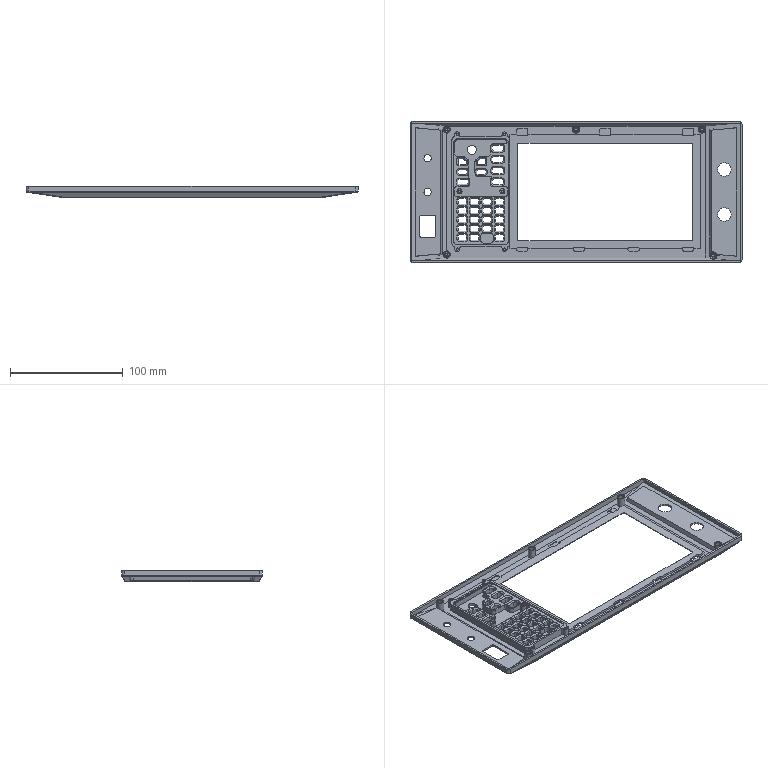NC program | NX | posted with a generic post | part box 295 x 125 x 10 mm
Lines 11539 to 12429 of 134431:
(HOLE_MILLING , TOOL : D4)
N23028 T04 M6
N23030 G54
N23032 G17 G0 G90 X-92.5 Y37.45 S9500 M3
N23034 G43 Z30. H4
N23036 Z-7.
N23038 G94 G3 X-91.875 Y36.825 R0.625 F1400.
N23040 X-91.25 Y37.45 R0.625
N23042 X-91.25 Y37.45 Z-7.4 I-1.25 J0.
N23044 X-91.25 Y37.45 Z-7.8 I-1.25 J0.
N23046 X-91.25 Y37.45 Z-8.2 I-1.25 J0.
N23048 X-91.25 Y37.45 Z-8.6 I-1.25 J0.
N23050 X-91.25 Y37.45 Z-9. I-1.25 J0.
N23052 X-91.25 Y37.45 Z-9.4 I-1.25 J0.
N23054 X-91.25 Y37.45 Z-9.8 I-1.25 J0.
N23056 X-93.75 Y37.45 Z-10. I-1.25 J0.
N23058 X-92.827 Y36.181 R1.334
N23060 X-91.326 Y36.665 R1.348
N23062 X-91.334 Y38.383 R1.44
N23064 X-93.103 Y38.905 R1.545
N23066 X-94.149 Y37.306 R1.602
N23068 X-92.839 Y35.746 R1.708
N23070 X-90.85 Y36.626 R1.798
N23072 X-91.156 Y38.794 R1.821
N23074 X-93.844 Y38.794 R1.9
N23076 X-91.156 Y38.794 R-1.9
N23078 X-92.5 Y38.794 R0.95
N23080 X-92.5 Y37.45 R0.95
N23082 G0 Z30.
N23084 X-131.817 Y30.
N23086 Z-3.769
N23088 G3 X-131.242 Y29.425 R0.575
N23090 X-130.667 Y30. R0.575
N23092 X-130.667 Y30. Z-4.169 I-1.15 J0.
N23094 X-130.667 Y30. Z-4.569 I-1.15 J0.
N23096 X-130.667 Y30. Z-4.969 I-1.15 J0.
N23098 X-130.667 Y30. Z-5.369 I-1.15 J0.
N23100 X-130.667 Y30. Z-5.769 I-1.15 J0.
N23102 X-131.817 Y31.15 R1.15
N23104 X-130.667 Y30. R-1.15
N23106 X-131.242 Y30.575 R0.575
N23108 X-131.817 Y30. R0.575
N23110 G0 Z30.
N23112 Y0.
N23114 Z-3.769
N23116 G3 X-131.242 Y-0.575 R0.575
N23118 X-130.667 Y0. R0.575
N23120 X-130.667 Y0. Z-4.169 I-1.15 J0.
N23122 X-130.667 Y0. Z-4.569 I-1.15 J0.
N23124 X-130.667 Y0. Z-4.969 I-1.15 J0.
N23126 X-130.667 Y0. Z-5.369 I-1.15 J0.
N23128 X-130.667 Y0. Z-5.769 I-1.15 J0.
N23130 X-131.817 Y1.15 R1.15
N23132 X-130.667 Y0. R-1.15
N23134 X-131.242 Y0.575 R0.575
N23136 X-131.817 Y0. R0.575
N23138 G0 Z30.
N23140 X131.817 Y20.
N23142 Z-3.769
N23144 G3 X132.442 Y19.375 R0.625
N23146 X133.067 Y20. R0.625
N23148 X133.067 Y20. Z-4.169 I-1.25 J0.
N23150 X133.067 Y20. Z-4.569 I-1.25 J0.
N23152 X133.067 Y20. Z-4.969 I-1.25 J0.
N23154 X133.067 Y20. Z-5.369 I-1.25 J0.
N23156 X133.067 Y20. Z-5.769 I-1.25 J0.
N23158 X131.862 Y21.318 R1.323
N23160 X130.398 Y20.241 R1.372
N23162 X131.41 Y18.522 R1.472
N23164 X133.354 Y19.462 R1.593
N23166 X132.543 Y21.562 R1.661
N23168 X130.226 Y20.879 R1.783
N23170 X130.734 Y18.424 R1.851
N23172 X133.386 Y18.749 R1.972
N23174 X133.278 Y21.51 R2.04
N23176 X130.353 Y21.638 R2.161
N23178 X129.972 Y18.642 R2.23
N23180 X133.086 Y17.98 R2.351
N23182 X134.031 Y21.116 R2.419
N23184 X130.831 Y22.379 R2.54
N23186 X129.266 Y19.213 R2.608
N23188 X132.432 Y17.305 R2.729
N23190 X134.651 Y20.375 R2.798
N23192 X131.651 Y22.949 R2.919
N23194 X128.771 Y20.11 R2.987
N23196 X131.465 Y16.877 R3.108
N23198 X134.987 Y19.345 R3.176
N23200 X132.739 Y23.202 R3.297
N23202 X128.624 Y21.245 R3.366
N23204 X130.289 Y16.827 R3.487
N23206 X134.919 Y18.142 R3.555
N23208 X133.964 Y23.026 R3.676
N23210 X128.846 Y22.427 R3.776
N23212 X129.059 Y17.242 R3.829
N23214 X134.575 Y17.242 R3.9
N23216 X129.059 Y17.242 R-3.9
N23218 X131.817 Y17.242 R1.95
N23220 X131.817 Y20. R1.95
N23222 G0 Z30.
N23224 Y-20.
N23226 Z-3.769
N23228 G3 X132.442 Y-20.625 R0.625
N23230 X133.067 Y-20. R0.625
N23232 X133.067 Y-20. Z-4.169 I-1.25 J0.
N23234 X133.067 Y-20. Z-4.569 I-1.25 J0.
N23236 X133.067 Y-20. Z-4.969 I-1.25 J0.
N23238 X133.067 Y-20. Z-5.369 I-1.25 J0.
N23240 X133.067 Y-20. Z-5.769 I-1.25 J0.
N23242 X131.862 Y-18.682 R1.323
N23244 X130.398 Y-19.759 R1.372
N23246 X131.41 Y-21.478 R1.472
N23248 X133.354 Y-20.538 R1.593
N23250 X132.543 Y-18.438 R1.661
N23252 X130.226 Y-19.121 R1.783
N23254 X130.734 Y-21.576 R1.851
N23256 X133.386 Y-21.251 R1.972
N23258 X133.278 Y-18.49 R2.04
N23260 X130.353 Y-18.362 R2.161
N23262 X129.972 Y-21.358 R2.23
N23264 X133.086 Y-22.02 R2.351
N23266 X134.031 Y-18.884 R2.419
N23268 X130.831 Y-17.621 R2.54
N23270 X129.266 Y-20.787 R2.608
N23272 X132.432 Y-22.695 R2.729
N23274 X134.651 Y-19.625 R2.798
N23276 X131.651 Y-17.051 R2.919
N23278 X128.771 Y-19.89 R2.987
N23280 X131.465 Y-23.123 R3.108
N23282 X134.987 Y-20.655 R3.176
N23284 X132.739 Y-16.798 R3.297
N23286 X128.624 Y-18.755 R3.366
N23288 X130.289 Y-23.173 R3.487
N23290 X134.919 Y-21.858 R3.555
N23292 X133.964 Y-16.974 R3.676
N23294 X128.846 Y-17.573 R3.776
N23296 X129.059 Y-22.758 R3.829
N23298 X134.575 Y-22.758 R3.9
N23300 X129.059 Y-22.758 R-3.9
N23302 X131.817 Y-22.758 R1.95
N23304 X131.817 Y-20. R1.95
N23306 G0 Z30.
(HOLE_MILLING_COPY , TOOL : D4)
N23308 X-92.5 Y37.45
N23310 Z-7.
N23312 G3 X-91.5 Y36.45 R1. F1000.
N23314 X-90.5 Y37.45 R1.
N23316 X-90.5 Y37.45 Z-9. I-2. J0.
N23318 X-94.5 Y37.45 Z-10. I-2. J0.
N23320 X-92.5 Y35.45 R2.
N23322 X-94.5 Y37.45 R-2.
N23324 X-93.5 Y36.45 R1.
N23326 X-92.5 Y37.45 R1.
N23328 G0 Z30.
N23330 X-131.817 Y30.
N23332 Z-3.769
N23334 G3 X-131.192 Y29.375 R0.625
N23336 X-130.567 Y30. R0.625
N23338 X-130.567 Y30. Z-5.769 I-1.25 J0.
N23340 X-131.817 Y31.25 R1.25
N23342 X-130.567 Y30. R-1.25
N23344 X-131.192 Y30.625 R0.625
N23346 X-131.817 Y30. R0.625
N23348 G0 Z30.
N23350 Y0.
N23352 Z-3.769
N23354 G3 X-131.192 Y-0.625 R0.625
N23356 X-130.567 Y0. R0.625
N23358 X-130.567 Y0. Z-5.769 I-1.25 J0.
N23360 X-131.817 Y1.25 R1.25
N23362 X-130.567 Y0. R-1.25
N23364 X-131.192 Y0.625 R0.625
N23366 X-131.817 Y0. R0.625
N23368 G0 Z30.
N23370 X131.817 Y20.
N23372 Z-3.769
N23374 G1 X132.202 Y19.187
N23376 G3 X135.817 Y20. R1.899
N23378 X135.817 Y20. Z-5.769 I-4. J0.
N23380 X131.817 Y24. R4.
N23382 X135.817 Y20. R-4.
N23384 X132.202 Y20.813 R1.899
N23386 G1 X131.817 Y20.
N23388 G0 Z30.
N23390 Y-20.
N23392 Z-3.769
N23394 G1 X132.202 Y-20.813
N23396 G3 X135.817 Y-20. R1.899
N23398 X135.817 Y-20. Z-5.769 I-4. J0.
N23400 X131.817 Y-16. R4.
N23402 X135.817 Y-20. R-4.
N23404 X132.202 Y-19.187 R1.899
N23406 G1 X131.817 Y-20.
N23408 G0 Z30.
(CAVITY_MILL_COPY_COPY , TOOL : D4)
N23410 X114.594 Y-58.2
N23412 Z0.625
N23414 G1 Z-0.375
N23416 X114.768 Y-58.5
N23418 G3 X115.634 Y-59. R1.
N23420 G1 X117.383 F1650.
N23422 G2 X116.837 Y-57.451 R5.25
N23424 G3 X116.188 Y-56.69 R1.
N23426 G1 X115.951 Y-56.606
N23428 Z0.625
N23430 G0 Z30.
N23432 X114.594 Y-58.2
N23434 Z0.25
N23436 G1 Z-0.75 F1000.
N23438 X114.768 Y-58.5
N23440 G3 X115.634 Y-59. R1.
N23442 G1 X117.383 F1650.
N23444 G2 X116.837 Y-57.451 R5.25
N23446 G3 X116.188 Y-56.69 R1.
N23448 G1 X115.951 Y-56.606
N23450 Z0.25
N23452 G0 X114.594 Y-58.2 Z-0.125
N23454 G1 Z-1.125 F1000.
N23456 X114.768 Y-58.5
N23458 G3 X115.634 Y-59. R1.
N23460 G1 X117.383 F1650.
N23462 G2 X116.837 Y-57.451 R5.25
N23464 G3 X116.188 Y-56.69 R1.
N23466 G1 X115.951 Y-56.606
N23468 Z-0.125
N23470 G0 X114.594 Y-58.2 Z-0.5
N23472 G1 Z-1.5 F1000.
N23474 X114.768 Y-58.5
N23476 G3 X115.634 Y-59. R1.
N23478 G1 X117.383 F1650.
N23480 G2 X116.837 Y-57.451 R5.25
N23482 G3 X116.188 Y-56.69 R1.
N23484 G1 X115.951 Y-56.606
N23486 Z-0.5
N23488 G0 X114.594 Y-58.2 Z-0.833
N23490 G1 Z-1.833 F1000.
N23492 X114.768 Y-58.5
N23494 G3 X115.634 Y-59. R1.
N23496 G1 X117.383 F1650.
N23498 G2 X116.837 Y-57.451 R5.25
N23500 G3 X116.188 Y-56.69 R1.
N23502 G1 X115.951 Y-56.606
N23504 Z-0.833
N23506 G0 X114.594 Y-58.2 Z-1.167
N23508 G1 Z-2.167 F1000.
N23510 X114.768 Y-58.5
N23512 G3 X115.634 Y-59. R1.
N23514 G1 X117.383 F1650.
N23516 G2 X116.837 Y-57.451 R5.25
N23518 G3 X116.188 Y-56.69 R1.
N23520 G1 X115.951 Y-56.606
N23522 Z-1.167
N23524 G0 X114.594 Y-58.2 Z-1.5
N23526 G1 Z-2.5 F1000.
N23528 X114.768 Y-58.5
N23530 G3 X115.634 Y-59. R1.
N23532 G1 X117.383 F1650.
N23534 G2 X116.837 Y-57.451 R5.25
N23536 G3 X116.188 Y-56.69 R1.
N23538 G1 X115.951 Y-56.606
N23540 Z-1.5
N23542 G0 X114.594 Y-58.2 Z-1.833
N23544 G1 Z-2.833 F1000.
N23546 X114.768 Y-58.5
N23548 G3 X115.634 Y-59. R1.
N23550 G1 X117.383 F1650.
N23552 G2 X116.837 Y-57.451 R5.25
N23554 G3 X116.188 Y-56.69 R1.
N23556 G1 X115.951 Y-56.606
N23558 Z-1.833
N23560 G0 X114.594 Y-58.2 Z-2.167
N23562 G1 Z-3.167 F1000.
N23564 X114.768 Y-58.5
N23566 G3 X115.634 Y-59. R1.
N23568 G1 X117.383 F1650.
N23570 G2 X116.837 Y-57.451 R5.25
N23572 G3 X116.188 Y-56.69 R1.
N23574 G1 X115.951 Y-56.606
N23576 Z-2.167
N23578 G0 X114.594 Y-58.2 Z-2.5
N23580 G1 Z-3.5 F1000.
N23582 X114.768 Y-58.5
N23584 G3 X115.634 Y-59. R1.
N23586 G1 X117.383 F1650.
N23588 G2 X116.837 Y-57.451 R5.25
N23590 G3 X116.188 Y-56.69 R1.
N23592 G1 X115.951 Y-56.606
N23594 Z-2.5
N23596 G0 X114.594 Y-58.2 Z-2.885
N23598 G1 Z-3.885 F1000.
N23600 X114.768 Y-58.5
N23602 G3 X115.634 Y-59. R1.
N23604 G1 X117.383 F1650.
N23606 G2 X116.837 Y-57.451 R5.25
N23608 G3 X116.188 Y-56.69 R1.
N23610 G1 X115.951 Y-56.606
N23612 Z-2.885
N23614 G0 X114.594 Y-58.2 Z-3.269
N23616 G1 Z-4.269 F1000.
N23618 X114.768 Y-58.5
N23620 G3 X115.634 Y-59. R1.
N23622 G1 X117.383 F1650.
N23624 G2 X116.837 Y-57.451 R5.25
N23626 G3 X116.188 Y-56.69 R1.
N23628 G1 X115.951 Y-56.606
N23630 Z-3.269
N23632 G0 X114.586 Y-58.166 Z-3.641
N23634 G1 Z-4.641 F1000.
N23636 X114.759 Y-58.466
N23638 G3 X115.625 Y-58.966 R1.
N23640 G1 X117.365 F1650.
N23642 G2 X116.832 Y-57.422 R5.25
N23644 G3 X116.187 Y-56.658 R1.
N23646 G1 X115.95 Y-56.572
N23648 Z-3.641
N23650 G0 X114.537 Y-57.943 Z-4.013
N23652 G1 Z-5.013 F1000.
N23654 X114.71 Y-58.243
N23656 G3 X115.576 Y-58.743 R1.
N23658 G1 X117.253 F1650.
N23660 G2 X116.801 Y-57.233 R5.25
N23662 G3 X116.185 Y-56.445 R1.
N23664 G1 X115.952 Y-56.351
N23666 Z-4.013
N23668 G0 X114.496 Y-57.72 Z-4.385
N23670 G1 Z-5.385 F1000.
N23672 X114.669 Y-58.02
N23674 G3 X115.535 Y-58.52 R1.
N23676 G1 X117.154 F1650.
N23678 G2 X116.778 Y-57.044 R5.25
N23680 G3 X116.191 Y-56.234 R1.
N23682 G1 X115.961 Y-56.131
N23684 Z-4.385
N23686 G0 X114.463 Y-57.497 Z-4.756
N23688 G1 Z-5.756 F1000.
N23690 X114.636 Y-57.797
N23692 G3 X115.502 Y-58.297 R1.
N23694 G1 X117.067 F1650.
N23696 G2 X116.762 Y-56.855 R5.25
N23698 G3 X116.205 Y-56.025 R1.
N23700 G1 X115.978 Y-55.914
N23702 Z-4.756
N23704 G0 X114.438 Y-57.274 Z-5.128
N23706 G1 Z-6.128 F1000.
N23708 X114.611 Y-57.574
N23710 G3 X115.477 Y-58.074 R1.
N23712 G1 X116.991 F1650.
N23714 G2 X116.753 Y-56.667 R5.25
N23716 G3 X116.225 Y-55.817 R1.
N23718 G1 X116.003 Y-55.698
N23720 Z-5.128
N23722 G0 X114.422 Y-57.052 Z-5.5
N23724 G1 Z-6.5 F1000.
N23726 X114.595 Y-57.352
N23728 G3 X115.461 Y-57.852 R1.
N23730 G1 X116.927 F1650.
N23732 G2 X116.75 Y-56.48 R5.25
N23734 G3 X116.253 Y-55.612 R1.
N23736 G1 X116.036 Y-55.485
N23738 Z-5.5
N23740 G0 X114.414 Y-56.851 Z-5.833
N23742 G1 Z-6.833 F1000.
N23744 X114.587 Y-57.151
N23746 G3 X115.453 Y-57.651 R1.
N23748 G1 X116.878 F1650.
N23750 G2 X116.753 Y-56.311 R5.25
N23752 G3 X116.285 Y-55.427 R1.
N23754 G1 X116.072 Y-55.293
N23756 Z-5.833
N23758 G0 X114.412 Y-56.651 Z-6.167
N23760 G1 Z-7.167 F1000.
N23762 X114.585 Y-56.951
N23764 G3 X115.451 Y-57.451 R1.
N23766 G1 X116.837 F1650.
N23768 G2 X116.762 Y-56.143 R5.25
N23770 G3 X116.322 Y-55.245 R1.
N23772 G1 X116.113 Y-55.104
N23774 Z-6.167
N23776 G0 X114.417 Y-56.452 Z-6.5
N23778 G1 Z-7.5 F1000.
N23780 X114.59 Y-56.752
N23782 G3 X115.456 Y-57.252 R1.
N23784 G1 X116.804 F1650.
N23786 G2 X116.776 Y-55.977 R5.25
N23788 G3 X116.365 Y-55.065 R1.
N23790 G1 X116.16 Y-54.918
N23792 Z-6.5
N23794 G0 X114.428 Y-56.251 Z-6.833
N23796 G1 Z-7.833 F1000.
N23798 X114.601 Y-56.551
N23800 G3 X115.467 Y-57.051 R1.
N23802 G1 X116.779 F1650.
N23804 G2 X116.796 Y-55.808 R5.25
N23806 G3 X116.414 Y-54.884 R1.
N23808 G1 X116.215 Y-54.73
N23810 Z-6.833
N23812 G0 X112.714 Y-56.051 Z-7.167
N23814 G1 Z-8.167 F1000.
N23816 X112.887 Y-56.351
N23818 G3 X113.753 Y-56.851 R1.
N23820 G1 X115.052 F1650.
N23822 Y-55.552
N23824 G3 X114.552 Y-54.686 R1.
N23826 G1 X114.252 Y-54.512
N23828 Z-7.167
N23830 G0 X110.563 Y-55.852 Z-7.5
N23832 G1 Z-8.5 F1000.
N23834 X110.737 Y-56.152
N23836 G3 X111.603 Y-56.652 R1.
N23838 G1 X112.902 F1650.
N23840 Y-55.353
N23842 G3 X112.402 Y-54.487 R1.
N23844 G1 X112.102 Y-54.314
N23846 Z-7.5
N23848 G0 Z30.
N23850 X116.397 Y-54.218
N23852 Z-3.641
N23854 G1 Z-4.641 F1000.
N23856 X116.649 Y-54.225
N23858 G3 X117.528 Y-53.749 R1.
N23860 G2 X117.883 Y-53.242 R5.25 F1650.
N23862 G1 Y-52.612
N23864 G3 X117.383 Y-51.746 R1.
N23866 G1 X117.083 Y-51.573
N23868 Z-3.641
N23870 G0 X116.334 Y-54.378 Z-4.013
N23872 G1 Z-5.013 F1000.
N23874 X116.586
N23876 G3 X117.452 Y-53.877 R1.
N23878 G2 X117.783 Y-53.372 R5.25 F1650.
N23880 G1 Y-52.759
N23882 G3 X117.283 Y-51.893 R1.
N23884 G1 X116.983 Y-51.719
N23886 Z-4.013
N23888 G0 X116.274 Y-54.546 Z-4.385
N23890 G1 Z-5.385 F1000.
N23892 X116.526 Y-54.539
N23894 G3 X117.376 Y-54.013 R1.
N23896 G2 X117.684 Y-53.511 R5.25 F1650.
N23898 G1 Y-52.915
N23900 G3 X117.184 Y-52.049 R1.
N23902 G1 X116.884 Y-51.875
N23904 Z-4.385
N23906 G0 X116.216 Y-54.725 Z-4.756
N23908 G1 Z-5.756 F1000.
N23910 X116.467 Y-54.71
N23912 G3 X117.301 Y-54.158 R1.
N23914 G2 X117.584 Y-53.66 R5.25 F1650.
N23916 G1 Y-53.082
N23918 G3 X117.084 Y-52.216 R1.
N23920 G1 X116.784 Y-52.042
N23922 Z-4.756
N23924 G0 X116.161 Y-54.917 Z-5.128
N23926 G1 Z-6.128 F1000.
N23928 X116.412 Y-54.893
N23930 G3 X117.227 Y-54.314 R1.
N23932 G2 X117.485 Y-53.822 R5.25 F1650.
N23934 G1 Y-53.261
N23936 G3 X116.985 Y-52.395 R1.
N23938 G1 X116.685 Y-52.222
N23940 Z-5.128
N23942 G0 X116.109 Y-55.121 Z-5.5
N23944 G1 Z-6.5 F1000.
N23946 X116.359 Y-55.088
N23948 G3 X117.154 Y-54.481 R1.
N23950 G2 X117.386 Y-53.996 R5.25 F1650.
N23952 G1 Y-53.455
N23954 G3 X116.886 Y-52.589 R1.
N23956 G1 X116.586 Y-52.416
N23958 Z-5.5
N23960 G0 X116.066 Y-55.321 Z-5.833
N23962 G1 Z-6.833 F1000.
N23964 X116.314 Y-55.281
N23966 G3 X117.088 Y-54.647 R1.
N23968 G2 X117.296 Y-54.17 R5.25 F1650.
N23970 G1 Y-53.647
N23972 G3 X116.796 Y-52.781 R1.
N23974 G1 X116.496 Y-52.608
N23976 Z-5.833
N23978 G0 X116.027 Y-55.539 Z-6.167
N23980 G1 Z-7.167 F1000.
N23982 X116.274 Y-55.489
N23984 G3 X117.024 Y-54.827 R1.
N23986 G2 X117.206 Y-54.359 R5.25 F1650.
N23988 G1 Y-53.857
N23990 G3 X116.706 Y-52.991 R1.
N23992 G1 X116.406 Y-52.818
N23994 Z-6.167
N23996 G0 Z30.
N23998 X128.049 Y-56.606
N24000 Z0.625
N24002 G1 Z-0.375 F1000.
N24004 X127.812 Y-56.69
N24006 G3 X127.163 Y-57.451 R1.
N24008 G2 X126.617 Y-59. R5.25 F1650.
N24010 G1 X128.366
N24012 G3 X129.232 Y-58.5 R1.
N24014 G1 X129.406 Y-58.2
N24016 Z0.625
N24018 G0 Z30.
N24020 X128.049 Y-56.606
N24022 Z0.25
N24024 G1 Z-0.75 F1000.
N24026 X127.812 Y-56.69
N24028 G3 X127.163 Y-57.451 R1.
N24030 G2 X126.617 Y-59. R5.25 F1650.
N24032 G1 X128.366
N24034 G3 X129.232 Y-58.5 R1.
N24036 G1 X129.406 Y-58.2
N24038 Z0.25
N24040 G0 X128.049 Y-56.606 Z-0.125
N24042 G1 Z-1.125 F1000.
N24044 X127.812 Y-56.69
N24046 G3 X127.163 Y-57.451 R1.
N24048 G2 X126.617 Y-59. R5.25 F1650.
N24050 G1 X128.366
N24052 G3 X129.232 Y-58.5 R1.
N24054 G1 X129.406 Y-58.2
N24056 Z-0.125
N24058 G0 X128.049 Y-56.606 Z-0.5
N24060 G1 Z-1.5 F1000.
N24062 X127.812 Y-56.69
N24064 G3 X127.163 Y-57.451 R1.
N24066 G2 X126.617 Y-59. R5.25 F1650.
N24068 G1 X128.366
N24070 G3 X129.232 Y-58.5 R1.
N24072 G1 X129.406 Y-58.2
N24074 Z-0.5
N24076 G0 X128.049 Y-56.606 Z-0.833
N24078 G1 Z-1.833 F1000.
N24080 X127.812 Y-56.69
N24082 G3 X127.163 Y-57.451 R1.
N24084 G2 X126.617 Y-59. R5.25 F1650.
N24086 G1 X128.366
N24088 G3 X129.232 Y-58.5 R1.
N24090 G1 X129.406 Y-58.2
N24092 Z-0.833
N24094 G0 X128.049 Y-56.606 Z-1.167
N24096 G1 Z-2.167 F1000.
N24098 X127.812 Y-56.69
N24100 G3 X127.163 Y-57.451 R1.
N24102 G2 X126.617 Y-59. R5.25 F1650.
N24104 G1 X128.366
N24106 G3 X129.232 Y-58.5 R1.
N24108 G1 X129.406 Y-58.2
N24110 Z-1.167
N24112 G0 X128.049 Y-56.606 Z-1.5
N24114 G1 Z-2.5 F1000.
N24116 X127.812 Y-56.69
N24118 G3 X127.163 Y-57.451 R1.
N24120 G2 X126.617 Y-59. R5.25 F1650.
N24122 G1 X128.366
N24124 G3 X129.232 Y-58.5 R1.
N24126 G1 X129.406 Y-58.2
N24128 Z-1.5
N24130 G0 X128.049 Y-56.606 Z-1.833
N24132 G1 Z-2.833 F1000.
N24134 X127.812 Y-56.69
N24136 G3 X127.163 Y-57.451 R1.
N24138 G2 X126.617 Y-59. R5.25 F1650.
N24140 G1 X128.366
N24142 G3 X129.232 Y-58.5 R1.
N24144 G1 X129.406 Y-58.2
N24146 Z-1.833
N24148 G0 X128.049 Y-56.606 Z-2.167
N24150 G1 Z-3.167 F1000.
N24152 X127.812 Y-56.69
N24154 G3 X127.163 Y-57.451 R1.
N24156 G2 X126.617 Y-59. R5.25 F1650.
N24158 G1 X128.366
N24160 G3 X129.232 Y-58.5 R1.
N24162 G1 X129.406 Y-58.2
N24164 Z-2.167
N24166 G0 X128.049 Y-56.606 Z-2.5
N24168 G1 Z-3.5 F1000.
N24170 X127.812 Y-56.69
N24172 G3 X127.163 Y-57.451 R1.
N24174 G2 X126.617 Y-59. R5.25 F1650.
N24176 G1 X128.366
N24178 G3 X129.232 Y-58.5 R1.
N24180 G1 X129.406 Y-58.2
N24182 Z-2.5
N24184 G0 X128.049 Y-56.606 Z-2.885
N24186 G1 Z-3.885 F1000.
N24188 X127.812 Y-56.69
N24190 G3 X127.163 Y-57.451 R1.
N24192 G2 X126.617 Y-59. R5.25 F1650.
N24194 G1 X128.366
N24196 G3 X129.232 Y-58.5 R1.
N24198 G1 X129.406 Y-58.2
N24200 Z-2.885
N24202 G0 X128.049 Y-56.606 Z-3.269
N24204 G1 Z-4.269 F1000.
N24206 X127.812 Y-56.69
N24208 G3 X127.163 Y-57.451 R1.
N24210 G2 X126.617 Y-59. R5.25 F1650.
N24212 G1 X128.366
N24214 G3 X129.232 Y-58.5 R1.
N24216 G1 X129.406 Y-58.2
N24218 Z-3.269
N24220 G0 X129.946 Y-58.966
N24222 G1 X137.969 Z-3.69 F1000.
N24224 Y-58.725 Z-3.702
N24226 X127.106 Y-57.722 Z-4.274
N24228 X127.03 Y-58.037 Z-4.291
N24230 X126.787 Y-58.68 Z-4.327
N24232 X126.635 Y-58.966 Z-4.344
N24234 X132.302 Z-4.641
N24236 X137.969 F1650.
N24238 Y-58.725
N24240 X127.106 Y-57.722
N24242 G2 X126.635 Y-58.966 R5.25
N24244 G1 X132.302
N24246 G3 X133.168 Y-58.466 R1.
N24248 G1 Z-3.641
N24250 G0 X129.422 Y-58.036
N24252 G1 X127.081 Y-57.82 Z-3.764 F1000.
N24254 X127. Y-58.134 Z-3.781
N24256 X126.885 Y-58.45 Z-3.799
N24258 X126.747 Y-58.743 Z-3.816
N24260 X135.552 Z-4.277
N24262 Y-58.602 Z-4.285
N24264 X127.081 Y-57.82 Z-4.73
N24266 X127. Y-58.134 Z-4.747
N24268 X126.885 Y-58.45 Z-4.765
N24270 X126.747 Y-58.743 Z-4.782
N24272 X131.149 Z-5.013
N24274 X135.552 F1650.
N24276 Y-58.602
N24278 X127.081 Y-57.82
N24280 G2 X126.747 Y-58.743 R5.25
N24282 G1 X131.149
N24284 G3 X131.582 Y-58.493 R0.5
N24286 G1 Z-4.013
N24288 G0 X129.966 Y-58.52
N24290 G1 X133.135 Z-4.179 F1000.
N24292 Y-58.479 Z-4.181
N24294 X127.055 Y-57.918 Z-4.501
N24296 X126.969 Y-58.225 Z-4.518
N24298 X126.846 Y-58.52 Z-4.535
N24300 X133.135 Z-4.864
N24302 Y-58.479 Z-4.866
N24304 X127.055 Y-57.918 Z-5.186
N24306 X126.969 Y-58.225 Z-5.203
N24308 X126.846 Y-58.52 Z-5.22
N24310 X129.991 Z-5.385
N24312 X133.135 F1650.
N24314 Y-58.479
N24316 X127.055 Y-57.918
N24318 G2 X126.846 Y-58.52 R5.25
N24320 G1 X129.991
N24322 G3 X130.424 Y-58.27 R0.5
N24324 G1 Z-4.385
N24326 G0 X128.374 Y-58.297
N24328 G1 X130.08 Z-4.474 F1000.
N24330 X127.027 Y-58.015 Z-4.635
N24332 X126.984 Y-58.157 Z-4.643
N24334 X126.933 Y-58.297 Z-4.65
N24336 X130.08 Z-4.815
N24338 X127.027 Y-58.015 Z-4.976
N24340 X126.984 Y-58.157 Z-4.984
N24342 X126.933 Y-58.297 Z-4.992
N24344 X130.08 Z-5.156
N24346 X127.027 Y-58.015 Z-5.317
N24348 X126.984 Y-58.157 Z-5.325
N24350 X126.933 Y-58.297 Z-5.333
N24352 X130.08 Z-5.498
N24354 X127.027 Y-58.015 Z-5.658
N24356 X126.984 Y-58.157 Z-5.666
N24358 X126.933 Y-58.297 Z-5.674
N24360 X128.506 Z-5.756
N24362 X130.08 F1650.
N24364 X127.027 Y-58.015
N24366 G2 X126.933 Y-58.297 R5.25
N24368 G1 X128.506
N24370 G3 X128.756 Y-58.23 R0.5
N24372 G1 Z-4.756
N24374 G0 Z30.
N24376 X141.662 Y-58.2
N24378 Z0.625
N24380 G1 Z-0.375 F1000.
N24382 X141.835 Y-58.5
N24384 G3 X142.701 Y-59. R1.
N24386 G1 X144. F1650.
N24388 Y-57.701
N24390 G3 X143.5 Y-56.835 R1.
N24392 G1 X143.2 Y-56.662
N24394 Z0.625
N24396 G0 Z30.
N24398 X141.662 Y-58.2
N24400 Z0.25
N24402 G1 Z-0.75 F1000.
N24404 X141.835 Y-58.5
N24406 G3 X142.701 Y-59. R1.
N24408 G1 X144. F1650.
N24410 Y-57.701
N24412 G3 X143.5 Y-56.835 R1.
N24414 G1 X143.2 Y-56.662
N24416 Z0.25
N24418 G0 X141.662 Y-58.2 Z-0.125
N24420 G1 Z-1.125 F1000.
N24422 X141.835 Y-58.5
N24424 G3 X142.701 Y-59. R1.
N24426 G1 X144. F1650.
N24428 Y-57.701
N24430 G3 X143.5 Y-56.835 R1.
N24432 G1 X143.2 Y-56.662
N24434 Z-0.125
N24436 G0 X141.662 Y-58.2 Z-0.5
N24438 G1 Z-1.5 F1000.
N24440 X141.835 Y-58.5
N24442 G3 X142.701 Y-59. R1.
N24444 G1 X144. F1650.
N24446 Y-57.701
N24448 G3 X143.5 Y-56.835 R1.
N24450 G1 X143.2 Y-56.662
N24452 Z-0.5
N24454 G0 X141.662 Y-58.2 Z-0.833
N24456 G1 Z-1.833 F1000.
N24458 X141.835 Y-58.5
N24460 G3 X142.701 Y-59. R1.
N24462 G1 X144. F1650.
N24464 Y-57.701
N24466 G3 X143.5 Y-56.835 R1.
N24468 G1 X143.2 Y-56.662
N24470 Z-0.833
N24472 G0 X141.662 Y-58.2 Z-1.167
N24474 G1 Z-2.167 F1000.
N24476 X141.835 Y-58.5
N24478 G3 X142.701 Y-59. R1.
N24480 G1 X144. F1650.
N24482 Y-57.701
N24484 G3 X143.5 Y-56.835 R1.
N24486 G1 X143.2 Y-56.662
N24488 Z-1.167
N24490 G0 X141.662 Y-58.2 Z-1.5
N24492 G1 Z-2.5 F1000.
N24494 X141.835 Y-58.5
N24496 G3 X142.701 Y-59. R1.
N24498 G1 X144. F1650.
N24500 Y-57.701
N24502 G3 X143.5 Y-56.835 R1.
N24504 G1 X143.2 Y-56.662
N24506 Z-1.5
N24508 G0 X141.662 Y-58.2 Z-1.833
N24510 G1 Z-2.833 F1000.
N24512 X141.835 Y-58.5
N24514 G3 X142.701 Y-59. R1.
N24516 G1 X144. F1650.
N24518 Y-57.701
N24520 G3 X143.5 Y-56.835 R1.
N24522 G1 X143.2 Y-56.662
N24524 Z-1.833
N24526 G0 X141.662 Y-58.2 Z-2.167
N24528 G1 Z-3.167 F1000.
N24530 X141.835 Y-58.5
N24532 G3 X142.701 Y-59. R1.
N24534 G1 X144. F1650.
N24536 Y-57.701
N24538 G3 X143.5 Y-56.835 R1.
N24540 G1 X143.2 Y-56.662
N24542 Z-2.167
N24544 G0 X141.662 Y-58.2 Z-2.5
N24546 G1 Z-3.5 F1000.
N24548 X141.835 Y-58.5
N24550 G3 X142.701 Y-59. R1.
N24552 G1 X144. F1650.
N24554 Y-57.701
N24556 G3 X143.5 Y-56.835 R1.
N24558 G1 X143.2 Y-56.662
N24560 Z-2.5
N24562 G0 X140.547 Y-58.2 Z-2.885
N24564 G1 Z-3.885 F1000.
N24566 X140.72 Y-58.5
N24568 G3 X141.586 Y-59. R1.
N24570 G1 X142.885 F1650.
N24572 Y-57.701
N24574 G3 X142.385 Y-56.835 R1.
N24576 G1 X142.085 Y-56.662
N24578 Z-2.885
N24580 G0 X138.063 Y-58.2 Z-3.269
N24582 G1 Z-4.269 F1000.
N24584 X138.237 Y-58.5
N24586 G3 X139.103 Y-59. R1.
N24588 G1 X140.402 F1650.
N24590 Y-57.701
N24592 G3 X139.902 Y-56.835 R1.
N24594 G1 X139.602 Y-56.662
N24596 Z-3.269
N24598 G0 Z30.
N24600 X103.114 Y-52.879
N24602 Z-5.833
N24604 G1 Z-6.833 F1000.
N24606 X103.168 Y-52.732
N24608 G3 X103. Y-51.746 R1.
N24610 G2 X102.604 Y-50.97 R2. F1650.
N24612 G1 X101.643
N24614 G3 X100.777 Y-51.47 R1.
N24616 G1 X100.604 Y-51.77
N24618 Z-5.833
N24620 G0 X103.114 Y-52.879 Z-6.167
N24622 G1 Z-7.167 F1000.
N24624 X103.168 Y-52.732
N24626 G3 X103. Y-51.746 R1.
N24628 G2 X102.604 Y-50.97 R2. F1650.
N24630 G1 X101.643
N24632 G3 X100.777 Y-51.47 R1.
N24634 G1 X100.604 Y-51.77
N24636 Z-6.167
N24638 G0 X103.114 Y-52.879 Z-6.5
N24640 G1 Z-7.5 F1000.
N24642 X103.168 Y-52.732
N24644 G3 X103. Y-51.746 R1.
N24646 G2 X102.604 Y-50.97 R2. F1650.
N24648 G1 X101.643
N24650 G3 X100.777 Y-51.47 R1.
N24652 G1 X100.604 Y-51.77
N24654 Z-6.5
N24656 G0 X103.114 Y-52.879 Z-6.833
N24658 G1 Z-7.833 F1000.
N24660 X103.168 Y-52.732
N24662 G3 X103. Y-51.746 R1.
N24664 G2 X102.604 Y-50.97 R2. F1650.
N24666 G1 X101.643
N24668 G3 X100.777 Y-51.47 R1.
N24670 G1 X100.604 Y-51.77
N24672 Z-6.833
N24674 G0 X103.114 Y-52.879 Z-7.167
N24676 G1 Z-8.167 F1000.
N24678 X103.168 Y-52.732
N24680 G3 X103. Y-51.746 R1.
N24682 G2 X102.604 Y-50.97 R2. F1650.
N24684 G1 X101.643
N24686 G3 X100.777 Y-51.47 R1.
N24688 G1 X100.604 Y-51.77
N24690 Z-7.167
N24692 G0 X103.114 Y-52.879 Z-7.5
N24694 G1 Z-8.5 F1000.
N24696 X103.168 Y-52.732
N24698 G3 X103. Y-51.746 R1.
N24700 G2 X102.604 Y-50.97 R2. F1650.
N24702 G1 X101.643
N24704 G3 X100.777 Y-51.47 R1.
N24706 G1 X100.604 Y-51.77
N24708 Z-7.5
N24710 G0 Z30.
N24712 X98.476
N24714 Z-5.833
N24716 G1 Z-6.833 F1000.
N24718 X98.303 Y-51.47
N24720 G3 X97.437 Y-50.97 R1.
N24722 G1 X96.476 F1650.
N24724 G2 X96.08 Y-51.746 R2.
N24726 G3 X95.912 Y-52.732 R1.
N24728 G1 X95.966 Y-52.879
N24730 Z-5.833
N24732 G0 X98.476 Y-51.77 Z-6.167
N24734 G1 Z-7.167 F1000.
N24736 X98.303 Y-51.47
N24738 G3 X97.437 Y-50.97 R1.
N24740 G1 X96.476 F1650.
N24742 G2 X96.08 Y-51.746 R2.
N24744 G3 X95.912 Y-52.732 R1.
N24746 G1 X95.966 Y-52.879
N24748 Z-6.167
N24750 G0 X98.476 Y-51.77 Z-6.5
N24752 G1 Z-7.5 F1000.
N24754 X98.303 Y-51.47
N24756 G3 X97.437 Y-50.97 R1.
N24758 G1 X96.476 F1650.
N24760 G2 X96.08 Y-51.746 R2.
N24762 G3 X95.912 Y-52.732 R1.
N24764 G1 X95.966 Y-52.879
N24766 Z-6.5
N24768 G0 X98.476 Y-51.77 Z-6.833
N24770 G1 Z-7.833 F1000.
N24772 X98.303 Y-51.47
N24774 G3 X97.437 Y-50.97 R1.
N24776 G1 X96.476 F1650.
N24778 G2 X96.08 Y-51.746 R2.
N24780 G3 X95.912 Y-52.732 R1.
N24782 G1 X95.966 Y-52.879
N24784 Z-6.833
N24786 G0 X98.476 Y-51.77 Z-7.167
N24788 G1 Z-8.167 F1000.
N24790 X98.303 Y-51.47